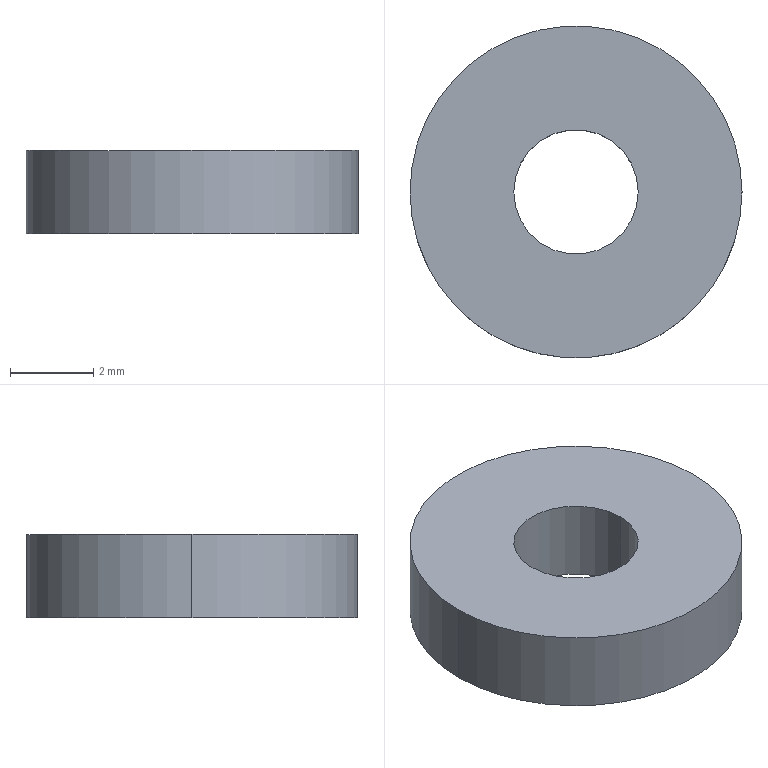Part | NX | 1 solid | 6 faces | box 8 x 8 x 2 mm | volume 86.394 mm3 | cylinder 4 | plane 2 | commonest cylinder face diameters 3 x2 8 x2
STEP:
#1=CARTESIAN_POINT('',(-4.,0.,-1.));
#2=VERTEX_POINT('',#1);
#3=CARTESIAN_POINT('',(4.,0.,-1.));
#4=VERTEX_POINT('',#3);
#5=CARTESIAN_POINT('',(0.,0.,-1.));
#6=DIRECTION('',(0.,0.,1.));
#7=DIRECTION('',(-1.,0.,0.));
#8=AXIS2_PLACEMENT_3D('',#5,#6,#7);
#9=CIRCLE('',#8,4.);
#10=EDGE_CURVE('',#2,#4,#9,.T.);
#11=ORIENTED_EDGE('',*,*,#10,.F.);
#12=CARTESIAN_POINT('',(0.,0.,-1.));
#13=DIRECTION('',(0.,0.,1.));
#14=DIRECTION('',(-1.,0.,0.));
#15=AXIS2_PLACEMENT_3D('',#12,#13,#14);
#16=CIRCLE('',#15,4.);
#17=EDGE_CURVE('',#4,#2,#16,.T.);
#18=ORIENTED_EDGE('',*,*,#17,.F.);
#19=EDGE_LOOP('',(#11,#18));
#20=FACE_BOUND('',#19,.T.);
#21=CARTESIAN_POINT('',(1.5,0.,-1.));
#22=VERTEX_POINT('',#21);
#23=CARTESIAN_POINT('',(-1.5,0.,-1.));
#24=VERTEX_POINT('',#23);
#25=CARTESIAN_POINT('',(0.,0.,-1.));
#26=DIRECTION('',(0.,0.,-1.));
#27=DIRECTION('',(-1.,0.,0.));
#28=AXIS2_PLACEMENT_3D('',#25,#26,#27);
#29=CIRCLE('',#28,1.5);
#30=EDGE_CURVE('',#22,#24,#29,.T.);
#31=ORIENTED_EDGE('',*,*,#30,.F.);
#32=CARTESIAN_POINT('',(0.,0.,-1.));
#33=DIRECTION('',(0.,0.,-1.));
#34=DIRECTION('',(-1.,0.,0.));
#35=AXIS2_PLACEMENT_3D('',#32,#33,#34);
#36=CIRCLE('',#35,1.5);
#37=EDGE_CURVE('',#24,#22,#36,.T.);
#38=ORIENTED_EDGE('',*,*,#37,.F.);
#39=EDGE_LOOP('',(#31,#38));
#40=FACE_BOUND('',#39,.T.);
#41=CARTESIAN_POINT('',(0.,0.,-1.));
#42=DIRECTION('',(0.,0.,1.));
#43=DIRECTION('',(1.,0.,0.));
#44=AXIS2_PLACEMENT_3D('',#41,#42,#43);
#45=PLANE('',#44);
#46=ADVANCED_FACE('',(#20,#40),#45,.F.);
#47=ORIENTED_EDGE('',*,*,#10,.T.);
#48=CARTESIAN_POINT('',(4.,0.,1.));
#49=VERTEX_POINT('',#48);
#50=CARTESIAN_POINT('',(4.,0.,-1.));
#51=DIRECTION('',(0.,0.,1.));
#52=VECTOR('',#51,1000.);
#53=LINE('',#50,#52);
#54=EDGE_CURVE('',#4,#49,#53,.T.);
#55=ORIENTED_EDGE('',*,*,#54,.T.);
#56=CARTESIAN_POINT('',(-4.,0.,1.));
#57=VERTEX_POINT('',#56);
#58=CARTESIAN_POINT('',(0.,0.,1.));
#59=DIRECTION('',(0.,0.,-1.));
#60=DIRECTION('',(-1.,0.,0.));
#61=AXIS2_PLACEMENT_3D('',#58,#59,#60);
#62=CIRCLE('',#61,4.);
#63=EDGE_CURVE('',#49,#57,#62,.T.);
#64=ORIENTED_EDGE('',*,*,#63,.T.);
#65=CARTESIAN_POINT('',(-4.,0.,-1.));
#66=DIRECTION('',(0.,0.,1.));
#67=VECTOR('',#66,1000.);
#68=LINE('',#65,#67);
#69=EDGE_CURVE('',#2,#57,#68,.T.);
#70=ORIENTED_EDGE('',*,*,#69,.F.);
#71=EDGE_LOOP('',(#47,#55,#64,#70));
#72=FACE_BOUND('',#71,.T.);
#73=CARTESIAN_POINT('',(0.,0.,-1.));
#74=DIRECTION('',(0.,0.,1.));
#75=DIRECTION('',(1.,0.,0.));
#76=AXIS2_PLACEMENT_3D('',#73,#74,#75);
#77=CYLINDRICAL_SURFACE('',#76,4.);
#78=ADVANCED_FACE('',(#72),#77,.T.);
#79=CARTESIAN_POINT('',(1.5,0.,1.));
#80=VERTEX_POINT('',#79);
#81=CARTESIAN_POINT('',(-1.5,0.,1.));
#82=VERTEX_POINT('',#81);
#83=CARTESIAN_POINT('',(0.,0.,1.));
#84=DIRECTION('',(0.,0.,1.));
#85=DIRECTION('',(1.,0.,0.));
#86=AXIS2_PLACEMENT_3D('',#83,#84,#85);
#87=CIRCLE('',#86,1.5);
#88=EDGE_CURVE('',#80,#82,#87,.T.);
#89=ORIENTED_EDGE('',*,*,#88,.T.);
#90=CARTESIAN_POINT('',(-1.5,0.,-1.));
#91=DIRECTION('',(0.,0.,1.));
#92=VECTOR('',#91,1000.);
#93=LINE('',#90,#92);
#94=EDGE_CURVE('',#82,#24,#93,.F.);
#95=ORIENTED_EDGE('',*,*,#94,.T.);
#96=ORIENTED_EDGE('',*,*,#37,.T.);
#97=CARTESIAN_POINT('',(1.5,0.,-1.));
#98=DIRECTION('',(0.,0.,1.));
#99=VECTOR('',#98,1000.);
#100=LINE('',#97,#99);
#101=EDGE_CURVE('',#80,#22,#100,.F.);
#102=ORIENTED_EDGE('',*,*,#101,.F.);
#103=EDGE_LOOP('',(#89,#95,#96,#102));
#104=FACE_BOUND('',#103,.T.);
#105=CARTESIAN_POINT('',(0.,0.,-1.));
#106=DIRECTION('',(0.,0.,1.));
#107=DIRECTION('',(1.,0.,0.));
#108=AXIS2_PLACEMENT_3D('',#105,#106,#107);
#109=CYLINDRICAL_SURFACE('',#108,1.5);
#110=ADVANCED_FACE('',(#104),#109,.F.);
#111=ORIENTED_EDGE('',*,*,#63,.F.);
#112=CARTESIAN_POINT('',(0.,0.,1.));
#113=DIRECTION('',(0.,0.,-1.));
#114=DIRECTION('',(-1.,0.,0.));
#115=AXIS2_PLACEMENT_3D('',#112,#113,#114);
#116=CIRCLE('',#115,4.);
#117=EDGE_CURVE('',#57,#49,#116,.T.);
#118=ORIENTED_EDGE('',*,*,#117,.F.);
#119=EDGE_LOOP('',(#111,#118));
#120=FACE_BOUND('',#119,.T.);
#121=ORIENTED_EDGE('',*,*,#88,.F.);
#122=CARTESIAN_POINT('',(0.,0.,1.));
#123=DIRECTION('',(0.,0.,1.));
#124=DIRECTION('',(1.,0.,0.));
#125=AXIS2_PLACEMENT_3D('',#122,#123,#124);
#126=CIRCLE('',#125,1.5);
#127=EDGE_CURVE('',#82,#80,#126,.T.);
#128=ORIENTED_EDGE('',*,*,#127,.F.);
#129=EDGE_LOOP('',(#121,#128));
#130=FACE_BOUND('',#129,.T.);
#131=CARTESIAN_POINT('',(0.,0.,1.));
#132=DIRECTION('',(0.,0.,1.));
#133=DIRECTION('',(1.,0.,0.));
#134=AXIS2_PLACEMENT_3D('',#131,#132,#133);
#135=PLANE('',#134);
#136=ADVANCED_FACE('',(#120,#130),#135,.T.);
#137=ORIENTED_EDGE('',*,*,#54,.F.);
#138=ORIENTED_EDGE('',*,*,#17,.T.);
#139=ORIENTED_EDGE('',*,*,#69,.T.);
#140=ORIENTED_EDGE('',*,*,#117,.T.);
#141=EDGE_LOOP('',(#137,#138,#139,#140));
#142=FACE_BOUND('',#141,.T.);
#143=CARTESIAN_POINT('',(0.,0.,-1.));
#144=DIRECTION('',(0.,0.,1.));
#145=DIRECTION('',(1.,0.,0.));
#146=AXIS2_PLACEMENT_3D('',#143,#144,#145);
#147=CYLINDRICAL_SURFACE('',#146,4.);
#148=ADVANCED_FACE('',(#142),#147,.T.);
#149=ORIENTED_EDGE('',*,*,#30,.T.);
#150=ORIENTED_EDGE('',*,*,#94,.F.);
#151=ORIENTED_EDGE('',*,*,#127,.T.);
#152=ORIENTED_EDGE('',*,*,#101,.T.);
#153=EDGE_LOOP('',(#149,#150,#151,#152));
#154=FACE_BOUND('',#153,.T.);
#155=CARTESIAN_POINT('',(0.,0.,-1.));
#156=DIRECTION('',(0.,0.,1.));
#157=DIRECTION('',(1.,0.,0.));
#158=AXIS2_PLACEMENT_3D('',#155,#156,#157);
#159=CYLINDRICAL_SURFACE('',#158,1.5);
#160=ADVANCED_FACE('',(#154),#159,.F.);
#161=CLOSED_SHELL('',(#46,#78,#110,#136,#148,#160));
#162=MANIFOLD_SOLID_BREP('',#161);
#163=(LENGTH_UNIT()NAMED_UNIT(*)SI_UNIT(.MILLI.,.METRE.));
#164=UNCERTAINTY_MEASURE_WITH_UNIT(LENGTH_MEASURE(0.00001),#163,'','');
#165=(NAMED_UNIT(*)PLANE_ANGLE_UNIT()SI_UNIT($,.RADIAN.));
#166=(NAMED_UNIT(*)SI_UNIT($,.STERADIAN.)SOLID_ANGLE_UNIT());
#167=(GEOMETRIC_REPRESENTATION_CONTEXT(3)GLOBAL_UNCERTAINTY_ASSIGNED_CONTEXT((#164))GLOBAL_UNIT_ASSIGNED_CONTEXT((#163,#165,#166))REPRESENTATION_CONTEXT('',''));
#168=ADVANCED_BREP_SHAPE_REPRESENTATION('',(#162),#167);